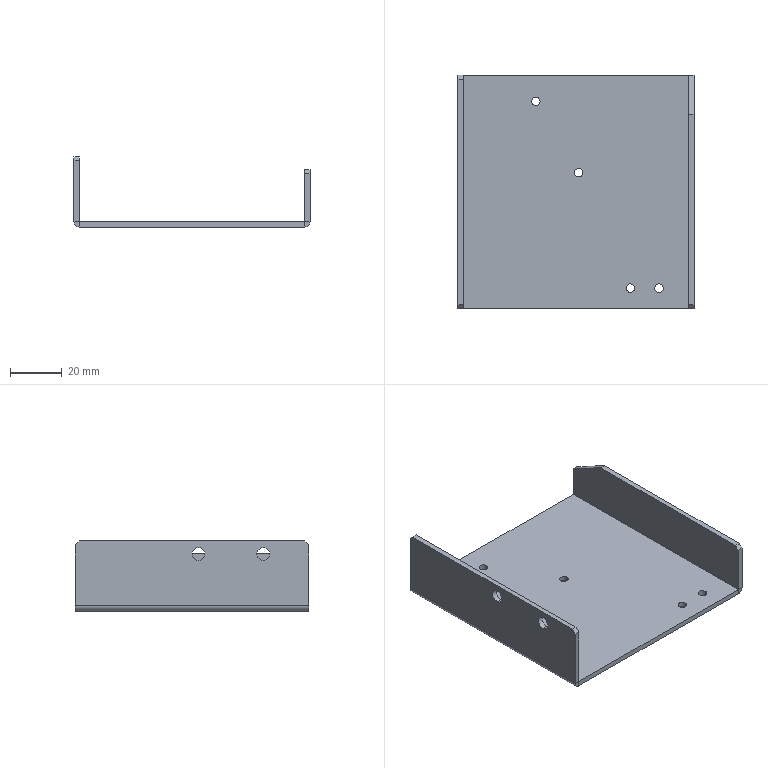Part | STEP file | drag chain fixing plate | 1 solid | 38 faces | box 91 x 90 x 27 mm | volume 24044 mm3 | plane 22 | cylinder 16 | commonest cylinder face diameters 3.3 x8 5 x4 0.1 x2 4.1 x2